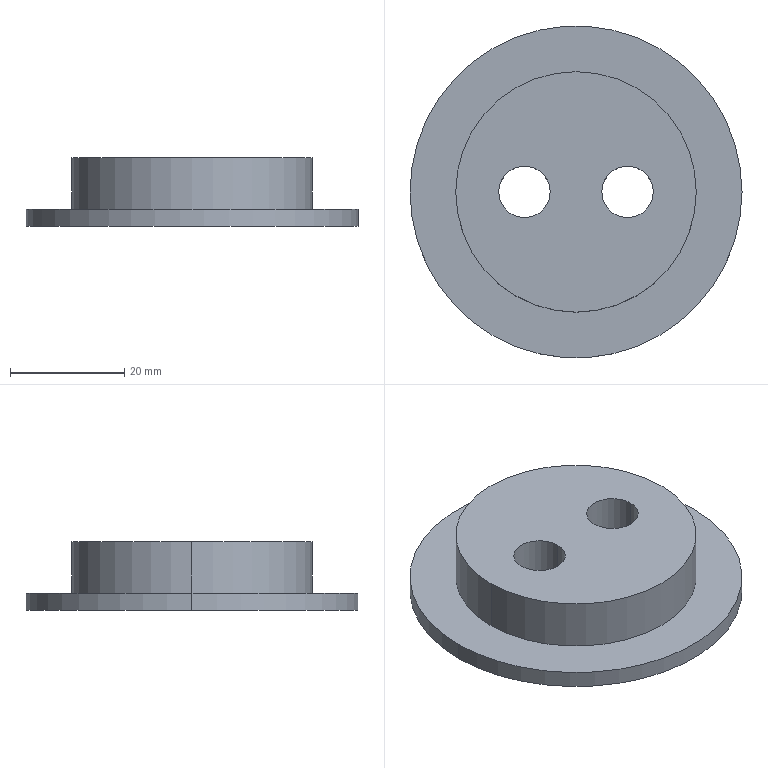Part | SolidWorks | features ICE 2, Extrusion 1 | 1 solid | 11 faces | box 58 x 58 x 12 mm | volume 18868 mm3 | cylinder 8 | plane 3 | commonest cylinder face diameters 9 x4 42 x2 58 x2
STEP:
#1=CARTESIAN_POINT('',(4.5,0.,0.));
#2=VERTEX_POINT('',#1);
#3=CARTESIAN_POINT('',(13.5,0.,0.));
#4=VERTEX_POINT('',#3);
#5=CARTESIAN_POINT('',(9.,0.,0.));
#6=DIRECTION('',(0.,0.,1.));
#7=DIRECTION('',(1.,0.,0.));
#8=AXIS2_PLACEMENT_3D('',#5,#6,#7);
#9=CIRCLE('',#8,4.5);
#10=EDGE_CURVE('',#2,#4,#9,.T.);
#11=ORIENTED_EDGE('',*,*,#10,.F.);
#12=CARTESIAN_POINT('',(4.5,0.,12.));
#13=VERTEX_POINT('',#12);
#14=CARTESIAN_POINT('',(4.5,0.,0.));
#15=DIRECTION('',(0.,0.,1.));
#16=VECTOR('',#15,1000.);
#17=LINE('',#14,#16);
#18=EDGE_CURVE('',#2,#13,#17,.T.);
#19=ORIENTED_EDGE('',*,*,#18,.T.);
#20=CARTESIAN_POINT('',(13.5,0.,12.));
#21=VERTEX_POINT('',#20);
#22=CARTESIAN_POINT('',(9.,0.,12.));
#23=DIRECTION('',(0.,0.,1.));
#24=DIRECTION('',(1.,0.,0.));
#25=AXIS2_PLACEMENT_3D('',#22,#23,#24);
#26=CIRCLE('',#25,4.5);
#27=EDGE_CURVE('',#13,#21,#26,.T.);
#28=ORIENTED_EDGE('',*,*,#27,.T.);
#29=CARTESIAN_POINT('',(13.5,0.,0.));
#30=DIRECTION('',(0.,0.,1.));
#31=VECTOR('',#30,1000.);
#32=LINE('',#29,#31);
#33=EDGE_CURVE('',#4,#21,#32,.T.);
#34=ORIENTED_EDGE('',*,*,#33,.F.);
#35=EDGE_LOOP('',(#11,#19,#28,#34));
#36=FACE_OUTER_BOUND('',#35,.T.);
#37=CARTESIAN_POINT('',(9.,0.,0.));
#38=DIRECTION('',(0.,0.,1.));
#39=DIRECTION('',(1.,0.,0.));
#40=AXIS2_PLACEMENT_3D('',#37,#38,#39);
#41=CYLINDRICAL_SURFACE('',#40,4.5);
#42=ADVANCED_FACE('',(#36),#41,.F.);
#43=CARTESIAN_POINT('',(-13.5,0.,0.));
#44=VERTEX_POINT('',#43);
#45=CARTESIAN_POINT('',(-4.5,0.,0.));
#46=VERTEX_POINT('',#45);
#47=CARTESIAN_POINT('',(-9.,0.,0.));
#48=DIRECTION('',(0.,0.,1.));
#49=DIRECTION('',(1.,0.,0.));
#50=AXIS2_PLACEMENT_3D('',#47,#48,#49);
#51=CIRCLE('',#50,4.5);
#52=EDGE_CURVE('',#44,#46,#51,.T.);
#53=ORIENTED_EDGE('',*,*,#52,.F.);
#54=CARTESIAN_POINT('',(-13.5,0.,12.));
#55=VERTEX_POINT('',#54);
#56=CARTESIAN_POINT('',(-13.5,0.,0.));
#57=DIRECTION('',(0.,0.,1.));
#58=VECTOR('',#57,1000.);
#59=LINE('',#56,#58);
#60=EDGE_CURVE('',#44,#55,#59,.T.);
#61=ORIENTED_EDGE('',*,*,#60,.T.);
#62=CARTESIAN_POINT('',(-4.5,0.,12.));
#63=VERTEX_POINT('',#62);
#64=CARTESIAN_POINT('',(-9.,0.,12.));
#65=DIRECTION('',(0.,0.,1.));
#66=DIRECTION('',(1.,0.,0.));
#67=AXIS2_PLACEMENT_3D('',#64,#65,#66);
#68=CIRCLE('',#67,4.5);
#69=EDGE_CURVE('',#55,#63,#68,.T.);
#70=ORIENTED_EDGE('',*,*,#69,.T.);
#71=CARTESIAN_POINT('',(-4.5,0.,0.));
#72=DIRECTION('',(0.,0.,1.));
#73=VECTOR('',#72,1000.);
#74=LINE('',#71,#73);
#75=EDGE_CURVE('',#46,#63,#74,.T.);
#76=ORIENTED_EDGE('',*,*,#75,.F.);
#77=EDGE_LOOP('',(#53,#61,#70,#76));
#78=FACE_OUTER_BOUND('',#77,.T.);
#79=CARTESIAN_POINT('',(-9.,0.,0.));
#80=DIRECTION('',(0.,0.,1.));
#81=DIRECTION('',(1.,0.,0.));
#82=AXIS2_PLACEMENT_3D('',#79,#80,#81);
#83=CYLINDRICAL_SURFACE('',#82,4.5);
#84=ADVANCED_FACE('',(#78),#83,.F.);
#85=CARTESIAN_POINT('',(21.,0.,12.));
#86=VERTEX_POINT('',#85);
#87=CARTESIAN_POINT('',(-21.,0.,12.));
#88=VERTEX_POINT('',#87);
#89=CARTESIAN_POINT('',(0.,0.,12.));
#90=DIRECTION('',(0.,0.,1.));
#91=DIRECTION('',(1.,0.,0.));
#92=AXIS2_PLACEMENT_3D('',#89,#90,#91);
#93=CIRCLE('',#92,21.);
#94=EDGE_CURVE('',#86,#88,#93,.T.);
#95=ORIENTED_EDGE('',*,*,#94,.F.);
#96=CARTESIAN_POINT('',(21.,0.,3.));
#97=VERTEX_POINT('',#96);
#98=CARTESIAN_POINT('',(21.,0.,12.));
#99=DIRECTION('',(0.,0.,-1.));
#100=VECTOR('',#99,1000.);
#101=LINE('',#98,#100);
#102=EDGE_CURVE('',#86,#97,#101,.T.);
#103=ORIENTED_EDGE('',*,*,#102,.T.);
#104=CARTESIAN_POINT('',(-21.,0.,3.));
#105=VERTEX_POINT('',#104);
#106=CARTESIAN_POINT('',(0.,0.,3.));
#107=DIRECTION('',(0.,0.,1.));
#108=DIRECTION('',(1.,0.,0.));
#109=AXIS2_PLACEMENT_3D('',#106,#107,#108);
#110=CIRCLE('',#109,21.);
#111=EDGE_CURVE('',#97,#105,#110,.T.);
#112=ORIENTED_EDGE('',*,*,#111,.T.);
#113=CARTESIAN_POINT('',(-21.,0.,12.));
#114=DIRECTION('',(0.,0.,-1.));
#115=VECTOR('',#114,1000.);
#116=LINE('',#113,#115);
#117=EDGE_CURVE('',#88,#105,#116,.T.);
#118=ORIENTED_EDGE('',*,*,#117,.F.);
#119=EDGE_LOOP('',(#95,#103,#112,#118));
#120=FACE_OUTER_BOUND('',#119,.T.);
#121=CARTESIAN_POINT('',(0.,0.,12.));
#122=DIRECTION('',(0.,0.,-1.));
#123=DIRECTION('',(-1.,0.,0.));
#124=AXIS2_PLACEMENT_3D('',#121,#122,#123);
#125=CYLINDRICAL_SURFACE('',#124,21.);
#126=ADVANCED_FACE('',(#120),#125,.T.);
#127=CARTESIAN_POINT('',(29.,0.,3.));
#128=VERTEX_POINT('',#127);
#129=CARTESIAN_POINT('',(-29.,0.,3.));
#130=VERTEX_POINT('',#129);
#131=CARTESIAN_POINT('',(0.,0.,3.));
#132=DIRECTION('',(0.,0.,1.));
#133=DIRECTION('',(1.,0.,0.));
#134=AXIS2_PLACEMENT_3D('',#131,#132,#133);
#135=CIRCLE('',#134,29.);
#136=EDGE_CURVE('',#128,#130,#135,.T.);
#137=ORIENTED_EDGE('',*,*,#136,.F.);
#138=CARTESIAN_POINT('',(29.,0.,0.));
#139=VERTEX_POINT('',#138);
#140=CARTESIAN_POINT('',(29.,0.,3.));
#141=DIRECTION('',(0.,0.,-1.));
#142=VECTOR('',#141,1000.);
#143=LINE('',#140,#142);
#144=EDGE_CURVE('',#128,#139,#143,.T.);
#145=ORIENTED_EDGE('',*,*,#144,.T.);
#146=CARTESIAN_POINT('',(-29.,0.,0.));
#147=VERTEX_POINT('',#146);
#148=CARTESIAN_POINT('',(0.,0.,0.));
#149=DIRECTION('',(0.,0.,1.));
#150=DIRECTION('',(1.,0.,0.));
#151=AXIS2_PLACEMENT_3D('',#148,#149,#150);
#152=CIRCLE('',#151,29.);
#153=EDGE_CURVE('',#139,#147,#152,.T.);
#154=ORIENTED_EDGE('',*,*,#153,.T.);
#155=CARTESIAN_POINT('',(-29.,0.,3.));
#156=DIRECTION('',(0.,0.,-1.));
#157=VECTOR('',#156,1000.);
#158=LINE('',#155,#157);
#159=EDGE_CURVE('',#130,#147,#158,.T.);
#160=ORIENTED_EDGE('',*,*,#159,.F.);
#161=EDGE_LOOP('',(#137,#145,#154,#160));
#162=FACE_OUTER_BOUND('',#161,.T.);
#163=CARTESIAN_POINT('',(0.,0.,3.));
#164=DIRECTION('',(0.,0.,-1.));
#165=DIRECTION('',(-1.,0.,0.));
#166=AXIS2_PLACEMENT_3D('',#163,#164,#165);
#167=CYLINDRICAL_SURFACE('',#166,29.);
#168=ADVANCED_FACE('',(#162),#167,.T.);
#169=CARTESIAN_POINT('',(0.,0.,3.));
#170=DIRECTION('',(0.,0.,1.));
#171=DIRECTION('',(1.,0.,0.));
#172=AXIS2_PLACEMENT_3D('',#169,#170,#171);
#173=CIRCLE('',#172,29.);
#174=EDGE_CURVE('',#130,#128,#173,.T.);
#175=ORIENTED_EDGE('',*,*,#174,.T.);
#176=ORIENTED_EDGE('',*,*,#136,.T.);
#177=EDGE_LOOP('',(#175,#176));
#178=FACE_OUTER_BOUND('',#177,.T.);
#179=CARTESIAN_POINT('',(0.,0.,3.));
#180=DIRECTION('',(0.,0.,1.));
#181=DIRECTION('',(1.,0.,0.));
#182=AXIS2_PLACEMENT_3D('',#179,#180,#181);
#183=CIRCLE('',#182,21.);
#184=EDGE_CURVE('',#105,#97,#183,.T.);
#185=ORIENTED_EDGE('',*,*,#184,.F.);
#186=ORIENTED_EDGE('',*,*,#111,.F.);
#187=EDGE_LOOP('',(#185,#186));
#188=FACE_BOUND('',#187,.T.);
#189=CARTESIAN_POINT('',(0.,0.,3.));
#190=DIRECTION('',(0.,0.,1.));
#191=DIRECTION('',(1.,0.,0.));
#192=AXIS2_PLACEMENT_3D('',#189,#190,#191);
#193=PLANE('',#192);
#194=ADVANCED_FACE('',(#178,#188),#193,.T.);
#195=ORIENTED_EDGE('',*,*,#144,.F.);
#196=ORIENTED_EDGE('',*,*,#174,.F.);
#197=ORIENTED_EDGE('',*,*,#159,.T.);
#198=CARTESIAN_POINT('',(0.,0.,0.));
#199=DIRECTION('',(0.,0.,1.));
#200=DIRECTION('',(1.,0.,0.));
#201=AXIS2_PLACEMENT_3D('',#198,#199,#200);
#202=CIRCLE('',#201,29.);
#203=EDGE_CURVE('',#147,#139,#202,.T.);
#204=ORIENTED_EDGE('',*,*,#203,.T.);
#205=EDGE_LOOP('',(#195,#196,#197,#204));
#206=FACE_OUTER_BOUND('',#205,.T.);
#207=CARTESIAN_POINT('',(0.,0.,3.));
#208=DIRECTION('',(0.,0.,-1.));
#209=DIRECTION('',(-1.,0.,0.));
#210=AXIS2_PLACEMENT_3D('',#207,#208,#209);
#211=CYLINDRICAL_SURFACE('',#210,29.);
#212=ADVANCED_FACE('',(#206),#211,.T.);
#213=CARTESIAN_POINT('',(9.,0.,0.));
#214=DIRECTION('',(0.,0.,1.));
#215=DIRECTION('',(1.,0.,0.));
#216=AXIS2_PLACEMENT_3D('',#213,#214,#215);
#217=CIRCLE('',#216,4.5);
#218=EDGE_CURVE('',#4,#2,#217,.T.);
#219=ORIENTED_EDGE('',*,*,#218,.T.);
#220=ORIENTED_EDGE('',*,*,#10,.T.);
#221=EDGE_LOOP('',(#219,#220));
#222=FACE_BOUND('',#221,.T.);
#223=CARTESIAN_POINT('',(-9.,0.,0.));
#224=DIRECTION('',(0.,0.,1.));
#225=DIRECTION('',(1.,0.,0.));
#226=AXIS2_PLACEMENT_3D('',#223,#224,#225);
#227=CIRCLE('',#226,4.5);
#228=EDGE_CURVE('',#46,#44,#227,.T.);
#229=ORIENTED_EDGE('',*,*,#228,.T.);
#230=ORIENTED_EDGE('',*,*,#52,.T.);
#231=EDGE_LOOP('',(#229,#230));
#232=FACE_BOUND('',#231,.T.);
#233=ORIENTED_EDGE('',*,*,#203,.F.);
#234=ORIENTED_EDGE('',*,*,#153,.F.);
#235=EDGE_LOOP('',(#233,#234));
#236=FACE_OUTER_BOUND('',#235,.T.);
#237=CARTESIAN_POINT('',(0.,0.,0.));
#238=DIRECTION('',(0.,0.,1.));
#239=DIRECTION('',(1.,0.,0.));
#240=AXIS2_PLACEMENT_3D('',#237,#238,#239);
#241=PLANE('',#240);
#242=ADVANCED_FACE('',(#222,#232,#236),#241,.F.);
#243=ORIENTED_EDGE('',*,*,#102,.F.);
#244=CARTESIAN_POINT('',(0.,0.,12.));
#245=DIRECTION('',(0.,0.,1.));
#246=DIRECTION('',(1.,0.,0.));
#247=AXIS2_PLACEMENT_3D('',#244,#245,#246);
#248=CIRCLE('',#247,21.);
#249=EDGE_CURVE('',#88,#86,#248,.T.);
#250=ORIENTED_EDGE('',*,*,#249,.F.);
#251=ORIENTED_EDGE('',*,*,#117,.T.);
#252=ORIENTED_EDGE('',*,*,#184,.T.);
#253=EDGE_LOOP('',(#243,#250,#251,#252));
#254=FACE_OUTER_BOUND('',#253,.T.);
#255=CARTESIAN_POINT('',(0.,0.,12.));
#256=DIRECTION('',(0.,0.,-1.));
#257=DIRECTION('',(-1.,0.,0.));
#258=AXIS2_PLACEMENT_3D('',#255,#256,#257);
#259=CYLINDRICAL_SURFACE('',#258,21.);
#260=ADVANCED_FACE('',(#254),#259,.T.);
#261=CARTESIAN_POINT('',(9.,0.,12.));
#262=DIRECTION('',(0.,0.,1.));
#263=DIRECTION('',(1.,0.,0.));
#264=AXIS2_PLACEMENT_3D('',#261,#262,#263);
#265=CIRCLE('',#264,4.5);
#266=EDGE_CURVE('',#21,#13,#265,.T.);
#267=ORIENTED_EDGE('',*,*,#266,.F.);
#268=ORIENTED_EDGE('',*,*,#27,.F.);
#269=EDGE_LOOP('',(#267,#268));
#270=FACE_BOUND('',#269,.T.);
#271=CARTESIAN_POINT('',(-9.,0.,12.));
#272=DIRECTION('',(0.,0.,1.));
#273=DIRECTION('',(1.,0.,0.));
#274=AXIS2_PLACEMENT_3D('',#271,#272,#273);
#275=CIRCLE('',#274,4.5);
#276=EDGE_CURVE('',#63,#55,#275,.T.);
#277=ORIENTED_EDGE('',*,*,#276,.F.);
#278=ORIENTED_EDGE('',*,*,#69,.F.);
#279=EDGE_LOOP('',(#277,#278));
#280=FACE_BOUND('',#279,.T.);
#281=ORIENTED_EDGE('',*,*,#249,.T.);
#282=ORIENTED_EDGE('',*,*,#94,.T.);
#283=EDGE_LOOP('',(#281,#282));
#284=FACE_OUTER_BOUND('',#283,.T.);
#285=CARTESIAN_POINT('',(0.,0.,12.));
#286=DIRECTION('',(0.,0.,1.));
#287=DIRECTION('',(1.,0.,0.));
#288=AXIS2_PLACEMENT_3D('',#285,#286,#287);
#289=PLANE('',#288);
#290=ADVANCED_FACE('',(#270,#280,#284),#289,.T.);
#291=ORIENTED_EDGE('',*,*,#60,.F.);
#292=ORIENTED_EDGE('',*,*,#228,.F.);
#293=ORIENTED_EDGE('',*,*,#75,.T.);
#294=ORIENTED_EDGE('',*,*,#276,.T.);
#295=EDGE_LOOP('',(#291,#292,#293,#294));
#296=FACE_OUTER_BOUND('',#295,.T.);
#297=CARTESIAN_POINT('',(-9.,0.,0.));
#298=DIRECTION('',(0.,0.,1.));
#299=DIRECTION('',(1.,0.,0.));
#300=AXIS2_PLACEMENT_3D('',#297,#298,#299);
#301=CYLINDRICAL_SURFACE('',#300,4.5);
#302=ADVANCED_FACE('',(#296),#301,.F.);
#303=ORIENTED_EDGE('',*,*,#18,.F.);
#304=ORIENTED_EDGE('',*,*,#218,.F.);
#305=ORIENTED_EDGE('',*,*,#33,.T.);
#306=ORIENTED_EDGE('',*,*,#266,.T.);
#307=EDGE_LOOP('',(#303,#304,#305,#306));
#308=FACE_OUTER_BOUND('',#307,.T.);
#309=CARTESIAN_POINT('',(9.,0.,0.));
#310=DIRECTION('',(0.,0.,1.));
#311=DIRECTION('',(1.,0.,0.));
#312=AXIS2_PLACEMENT_3D('',#309,#310,#311);
#313=CYLINDRICAL_SURFACE('',#312,4.5);
#314=ADVANCED_FACE('',(#308),#313,.F.);
#315=CLOSED_SHELL('',(#42,#84,#126,#168,#194,#212,#242,#260,#290,#302,#314));
#316=MANIFOLD_SOLID_BREP('',#315);
#317=CARTESIAN_POINT('',(0.,0.,0.));
#318=DIRECTION('',(0.,0.,1.));
#319=DIRECTION('',(1.,0.,0.));
#320=AXIS2_PLACEMENT_3D('',#317,#318,#319);
#321=(LENGTH_UNIT()NAMED_UNIT(*)SI_UNIT(.MILLI.,.METRE.));
#322=UNCERTAINTY_MEASURE_WITH_UNIT(LENGTH_MEASURE(0.00001),#321,'','');
#323=(NAMED_UNIT(*)PLANE_ANGLE_UNIT()SI_UNIT($,.RADIAN.));
#324=(NAMED_UNIT(*)SI_UNIT($,.STERADIAN.)SOLID_ANGLE_UNIT());
#325=(GEOMETRIC_REPRESENTATION_CONTEXT(3)GLOBAL_UNCERTAINTY_ASSIGNED_CONTEXT((#322))GLOBAL_UNIT_ASSIGNED_CONTEXT((#321,#323,#324))REPRESENTATION_CONTEXT('',''));
#326=ADVANCED_BREP_SHAPE_REPRESENTATION('',(#316,#320),#325);